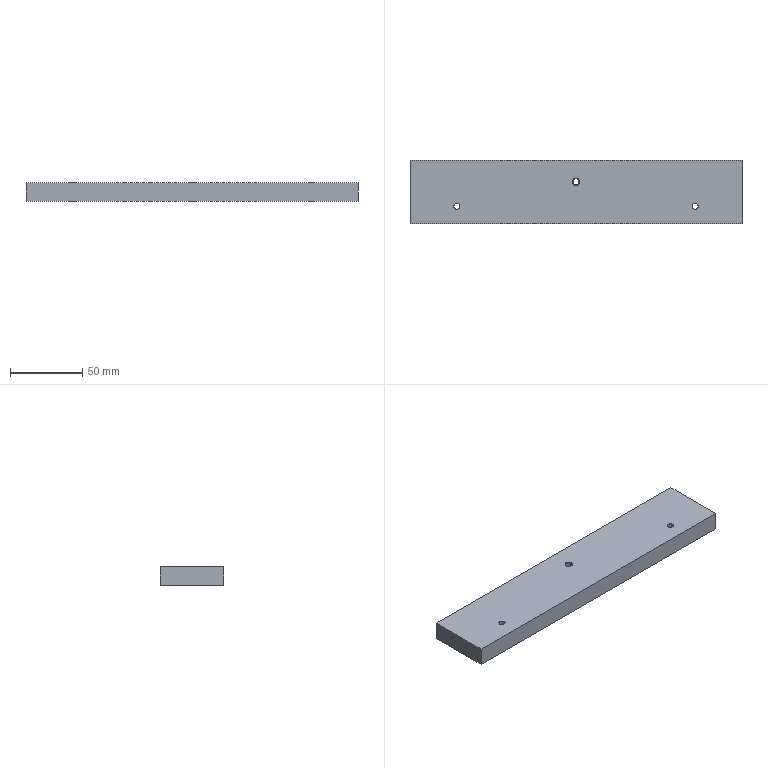Part | STEP file | A14-019 | 1 solid | 38 faces | box 230 x 44 x 13 mm | volume 129953 mm3 | cylinder 18 | cone 14 | plane 6 | commonest cylinder face diameters 4.2 x18